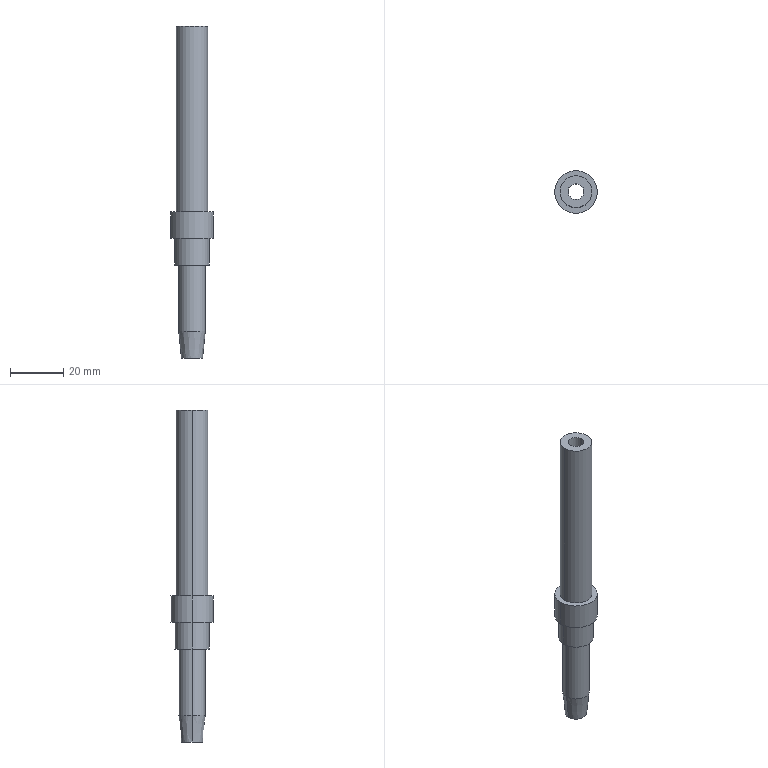Part | SolidWorks | features ICE 3, Chamfer 1, Extrusion 1 | 1 solid | 17 faces | box 16 x 16 x 125 mm | volume 10323 mm3 | cylinder 10 | plane 5 | cone 2 | commonest cylinder face diameters 6 x2 10 x2 12 x2 13 x2 16 x2
STEP:
#1=CARTESIAN_POINT('',(-4.,0.,0.));
#2=VERTEX_POINT('',#1);
#3=CARTESIAN_POINT('',(4.,0.,0.));
#4=VERTEX_POINT('',#3);
#5=CARTESIAN_POINT('',(0.,0.,0.));
#6=DIRECTION('',(0.,0.,-1.));
#7=DIRECTION('',(1.,0.,0.));
#8=AXIS2_PLACEMENT_3D('',#5,#6,#7);
#9=CIRCLE('',#8,4.);
#10=EDGE_CURVE('',#2,#4,#9,.T.);
#11=ORIENTED_EDGE('',*,*,#10,.F.);
#12=CARTESIAN_POINT('',(-5.,0.,10.));
#13=VERTEX_POINT('',#12);
#14=CARTESIAN_POINT('',(-5.,0.,10.));
#15=DIRECTION('',(-0.0995,0.,0.995));
#16=VECTOR('',#15,1000.);
#17=LINE('',#14,#16);
#18=EDGE_CURVE('',#2,#13,#17,.T.);
#19=ORIENTED_EDGE('',*,*,#18,.T.);
#20=CARTESIAN_POINT('',(5.,0.,10.));
#21=VERTEX_POINT('',#20);
#22=CARTESIAN_POINT('',(0.,0.,10.));
#23=DIRECTION('',(0.,0.,1.));
#24=DIRECTION('',(1.,0.,0.));
#25=AXIS2_PLACEMENT_3D('',#22,#23,#24);
#26=CIRCLE('',#25,5.);
#27=EDGE_CURVE('',#21,#13,#26,.T.);
#28=ORIENTED_EDGE('',*,*,#27,.F.);
#29=CARTESIAN_POINT('',(5.,0.,10.));
#30=DIRECTION('',(0.0995,0.,0.995));
#31=VECTOR('',#30,1000.);
#32=LINE('',#29,#31);
#33=EDGE_CURVE('',#4,#21,#32,.T.);
#34=ORIENTED_EDGE('',*,*,#33,.F.);
#35=EDGE_LOOP('',(#11,#19,#28,#34));
#36=FACE_OUTER_BOUND('',#35,.T.);
#37=CARTESIAN_POINT('',(0.,0.,10.));
#38=DIRECTION('',(0.,0.,1.));
#39=DIRECTION('',(1.,0.,0.));
#40=AXIS2_PLACEMENT_3D('',#37,#38,#39);
#41=CONICAL_SURFACE('',#40,5.,0.09967);
#42=ADVANCED_FACE('',(#36),#41,.T.);
#43=CARTESIAN_POINT('',(6.,0.,125.));
#44=VERTEX_POINT('',#43);
#45=CARTESIAN_POINT('',(-6.,0.,125.));
#46=VERTEX_POINT('',#45);
#47=CARTESIAN_POINT('',(0.,0.,125.));
#48=DIRECTION('',(0.,0.,1.));
#49=DIRECTION('',(1.,0.,0.));
#50=AXIS2_PLACEMENT_3D('',#47,#48,#49);
#51=CIRCLE('',#50,6.);
#52=EDGE_CURVE('',#44,#46,#51,.T.);
#53=ORIENTED_EDGE('',*,*,#52,.F.);
#54=CARTESIAN_POINT('',(6.,0.,55.));
#55=VERTEX_POINT('',#54);
#56=CARTESIAN_POINT('',(6.,0.,125.));
#57=DIRECTION('',(0.,0.,-1.));
#58=VECTOR('',#57,1000.);
#59=LINE('',#56,#58);
#60=EDGE_CURVE('',#44,#55,#59,.T.);
#61=ORIENTED_EDGE('',*,*,#60,.T.);
#62=CARTESIAN_POINT('',(-6.,0.,55.));
#63=VERTEX_POINT('',#62);
#64=CARTESIAN_POINT('',(0.,0.,55.));
#65=DIRECTION('',(0.,0.,1.));
#66=DIRECTION('',(1.,0.,0.));
#67=AXIS2_PLACEMENT_3D('',#64,#65,#66);
#68=CIRCLE('',#67,6.);
#69=EDGE_CURVE('',#55,#63,#68,.T.);
#70=ORIENTED_EDGE('',*,*,#69,.T.);
#71=CARTESIAN_POINT('',(-6.,0.,125.));
#72=DIRECTION('',(0.,0.,-1.));
#73=VECTOR('',#72,1000.);
#74=LINE('',#71,#73);
#75=EDGE_CURVE('',#46,#63,#74,.T.);
#76=ORIENTED_EDGE('',*,*,#75,.F.);
#77=EDGE_LOOP('',(#53,#61,#70,#76));
#78=FACE_OUTER_BOUND('',#77,.T.);
#79=CARTESIAN_POINT('',(0.,0.,125.));
#80=DIRECTION('',(0.,0.,-1.));
#81=DIRECTION('',(-1.,0.,0.));
#82=AXIS2_PLACEMENT_3D('',#79,#80,#81);
#83=CYLINDRICAL_SURFACE('',#82,6.);
#84=ADVANCED_FACE('',(#78),#83,.T.);
#85=CARTESIAN_POINT('',(8.,0.,55.));
#86=VERTEX_POINT('',#85);
#87=CARTESIAN_POINT('',(-8.,0.,55.));
#88=VERTEX_POINT('',#87);
#89=CARTESIAN_POINT('',(0.,0.,55.));
#90=DIRECTION('',(0.,0.,1.));
#91=DIRECTION('',(1.,0.,0.));
#92=AXIS2_PLACEMENT_3D('',#89,#90,#91);
#93=CIRCLE('',#92,8.);
#94=EDGE_CURVE('',#86,#88,#93,.T.);
#95=ORIENTED_EDGE('',*,*,#94,.F.);
#96=CARTESIAN_POINT('',(8.,0.,45.));
#97=VERTEX_POINT('',#96);
#98=CARTESIAN_POINT('',(8.,0.,55.));
#99=DIRECTION('',(0.,0.,-1.));
#100=VECTOR('',#99,1000.);
#101=LINE('',#98,#100);
#102=EDGE_CURVE('',#86,#97,#101,.T.);
#103=ORIENTED_EDGE('',*,*,#102,.T.);
#104=CARTESIAN_POINT('',(-8.,0.,45.));
#105=VERTEX_POINT('',#104);
#106=CARTESIAN_POINT('',(0.,0.,45.));
#107=DIRECTION('',(0.,0.,1.));
#108=DIRECTION('',(1.,0.,0.));
#109=AXIS2_PLACEMENT_3D('',#106,#107,#108);
#110=CIRCLE('',#109,8.);
#111=EDGE_CURVE('',#97,#105,#110,.T.);
#112=ORIENTED_EDGE('',*,*,#111,.T.);
#113=CARTESIAN_POINT('',(-8.,0.,55.));
#114=DIRECTION('',(0.,0.,-1.));
#115=VECTOR('',#114,1000.);
#116=LINE('',#113,#115);
#117=EDGE_CURVE('',#88,#105,#116,.T.);
#118=ORIENTED_EDGE('',*,*,#117,.F.);
#119=EDGE_LOOP('',(#95,#103,#112,#118));
#120=FACE_OUTER_BOUND('',#119,.T.);
#121=CARTESIAN_POINT('',(0.,0.,55.));
#122=DIRECTION('',(0.,0.,-1.));
#123=DIRECTION('',(-1.,0.,0.));
#124=AXIS2_PLACEMENT_3D('',#121,#122,#123);
#125=CYLINDRICAL_SURFACE('',#124,8.);
#126=ADVANCED_FACE('',(#120),#125,.T.);
#127=CARTESIAN_POINT('',(6.5,0.,45.));
#128=VERTEX_POINT('',#127);
#129=CARTESIAN_POINT('',(-6.5,0.,45.));
#130=VERTEX_POINT('',#129);
#131=CARTESIAN_POINT('',(0.,0.,45.));
#132=DIRECTION('',(0.,0.,1.));
#133=DIRECTION('',(1.,0.,0.));
#134=AXIS2_PLACEMENT_3D('',#131,#132,#133);
#135=CIRCLE('',#134,6.5);
#136=EDGE_CURVE('',#128,#130,#135,.T.);
#137=ORIENTED_EDGE('',*,*,#136,.F.);
#138=CARTESIAN_POINT('',(6.5,0.,35.));
#139=VERTEX_POINT('',#138);
#140=CARTESIAN_POINT('',(6.5,0.,45.));
#141=DIRECTION('',(0.,0.,-1.));
#142=VECTOR('',#141,1000.);
#143=LINE('',#140,#142);
#144=EDGE_CURVE('',#128,#139,#143,.T.);
#145=ORIENTED_EDGE('',*,*,#144,.T.);
#146=CARTESIAN_POINT('',(-6.5,0.,35.));
#147=VERTEX_POINT('',#146);
#148=CARTESIAN_POINT('',(0.,0.,35.));
#149=DIRECTION('',(0.,0.,1.));
#150=DIRECTION('',(1.,0.,0.));
#151=AXIS2_PLACEMENT_3D('',#148,#149,#150);
#152=CIRCLE('',#151,6.5);
#153=EDGE_CURVE('',#139,#147,#152,.T.);
#154=ORIENTED_EDGE('',*,*,#153,.T.);
#155=CARTESIAN_POINT('',(-6.5,0.,45.));
#156=DIRECTION('',(0.,0.,-1.));
#157=VECTOR('',#156,1000.);
#158=LINE('',#155,#157);
#159=EDGE_CURVE('',#130,#147,#158,.T.);
#160=ORIENTED_EDGE('',*,*,#159,.F.);
#161=EDGE_LOOP('',(#137,#145,#154,#160));
#162=FACE_OUTER_BOUND('',#161,.T.);
#163=CARTESIAN_POINT('',(0.,0.,45.));
#164=DIRECTION('',(0.,0.,-1.));
#165=DIRECTION('',(-1.,0.,0.));
#166=AXIS2_PLACEMENT_3D('',#163,#164,#165);
#167=CYLINDRICAL_SURFACE('',#166,6.5);
#168=ADVANCED_FACE('',(#162),#167,.T.);
#169=CARTESIAN_POINT('',(-3.,0.,125.));
#170=VERTEX_POINT('',#169);
#171=CARTESIAN_POINT('',(3.,0.,125.));
#172=VERTEX_POINT('',#171);
#173=CARTESIAN_POINT('',(0.,0.,125.));
#174=DIRECTION('',(0.,0.,1.));
#175=DIRECTION('',(1.,0.,0.));
#176=AXIS2_PLACEMENT_3D('',#173,#174,#175);
#177=CIRCLE('',#176,3.);
#178=EDGE_CURVE('',#170,#172,#177,.T.);
#179=ORIENTED_EDGE('',*,*,#178,.T.);
#180=CARTESIAN_POINT('',(3.,0.,0.));
#181=VERTEX_POINT('',#180);
#182=CARTESIAN_POINT('',(3.,0.,35.));
#183=DIRECTION('',(0.,0.,-1.));
#184=VECTOR('',#183,1000.);
#185=LINE('',#182,#184);
#186=EDGE_CURVE('',#172,#181,#185,.T.);
#187=ORIENTED_EDGE('',*,*,#186,.T.);
#188=CARTESIAN_POINT('',(-3.,0.,0.));
#189=VERTEX_POINT('',#188);
#190=CARTESIAN_POINT('',(0.,0.,0.));
#191=DIRECTION('',(0.,0.,1.));
#192=DIRECTION('',(1.,0.,0.));
#193=AXIS2_PLACEMENT_3D('',#190,#191,#192);
#194=CIRCLE('',#193,3.);
#195=EDGE_CURVE('',#189,#181,#194,.T.);
#196=ORIENTED_EDGE('',*,*,#195,.F.);
#197=CARTESIAN_POINT('',(-3.,0.,35.));
#198=DIRECTION('',(0.,0.,-1.));
#199=VECTOR('',#198,1000.);
#200=LINE('',#197,#199);
#201=EDGE_CURVE('',#170,#189,#200,.T.);
#202=ORIENTED_EDGE('',*,*,#201,.F.);
#203=EDGE_LOOP('',(#179,#187,#196,#202));
#204=FACE_OUTER_BOUND('',#203,.T.);
#205=CARTESIAN_POINT('',(0.,0.,35.));
#206=DIRECTION('',(0.,0.,-1.));
#207=DIRECTION('',(-1.,0.,0.));
#208=AXIS2_PLACEMENT_3D('',#205,#206,#207);
#209=CYLINDRICAL_SURFACE('',#208,3.);
#210=ADVANCED_FACE('',(#204),#209,.F.);
#211=CARTESIAN_POINT('',(5.,0.,35.));
#212=VERTEX_POINT('',#211);
#213=CARTESIAN_POINT('',(-5.,0.,35.));
#214=VERTEX_POINT('',#213);
#215=CARTESIAN_POINT('',(0.,0.,35.));
#216=DIRECTION('',(0.,0.,1.));
#217=DIRECTION('',(1.,0.,0.));
#218=AXIS2_PLACEMENT_3D('',#215,#216,#217);
#219=CIRCLE('',#218,5.);
#220=EDGE_CURVE('',#212,#214,#219,.T.);
#221=ORIENTED_EDGE('',*,*,#220,.F.);
#222=CARTESIAN_POINT('',(5.,0.,35.));
#223=DIRECTION('',(0.,0.,-1.));
#224=VECTOR('',#223,1000.);
#225=LINE('',#222,#224);
#226=EDGE_CURVE('',#212,#21,#225,.T.);
#227=ORIENTED_EDGE('',*,*,#226,.T.);
#228=ORIENTED_EDGE('',*,*,#27,.T.);
#229=CARTESIAN_POINT('',(-5.,0.,35.));
#230=DIRECTION('',(0.,0.,-1.));
#231=VECTOR('',#230,1000.);
#232=LINE('',#229,#231);
#233=EDGE_CURVE('',#214,#13,#232,.T.);
#234=ORIENTED_EDGE('',*,*,#233,.F.);
#235=EDGE_LOOP('',(#221,#227,#228,#234));
#236=FACE_OUTER_BOUND('',#235,.T.);
#237=CARTESIAN_POINT('',(0.,0.,35.));
#238=DIRECTION('',(0.,0.,-1.));
#239=DIRECTION('',(-1.,0.,0.));
#240=AXIS2_PLACEMENT_3D('',#237,#238,#239);
#241=CYLINDRICAL_SURFACE('',#240,5.);
#242=ADVANCED_FACE('',(#236),#241,.T.);
#243=CARTESIAN_POINT('',(0.,0.,0.));
#244=DIRECTION('',(0.,0.,-1.));
#245=DIRECTION('',(1.,0.,0.));
#246=AXIS2_PLACEMENT_3D('',#243,#244,#245);
#247=CIRCLE('',#246,4.);
#248=EDGE_CURVE('',#4,#2,#247,.T.);
#249=ORIENTED_EDGE('',*,*,#248,.T.);
#250=ORIENTED_EDGE('',*,*,#10,.T.);
#251=EDGE_LOOP('',(#249,#250));
#252=FACE_OUTER_BOUND('',#251,.T.);
#253=ORIENTED_EDGE('',*,*,#195,.T.);
#254=CARTESIAN_POINT('',(0.,0.,0.));
#255=DIRECTION('',(0.,0.,1.));
#256=DIRECTION('',(1.,0.,0.));
#257=AXIS2_PLACEMENT_3D('',#254,#255,#256);
#258=CIRCLE('',#257,3.);
#259=EDGE_CURVE('',#181,#189,#258,.T.);
#260=ORIENTED_EDGE('',*,*,#259,.T.);
#261=EDGE_LOOP('',(#253,#260));
#262=FACE_BOUND('',#261,.T.);
#263=CARTESIAN_POINT('',(0.,0.,0.));
#264=DIRECTION('',(0.,0.,1.));
#265=DIRECTION('',(1.,0.,0.));
#266=AXIS2_PLACEMENT_3D('',#263,#264,#265);
#267=PLANE('',#266);
#268=ADVANCED_FACE('',(#252,#262),#267,.F.);
#269=ORIENTED_EDGE('',*,*,#226,.F.);
#270=CARTESIAN_POINT('',(0.,0.,35.));
#271=DIRECTION('',(0.,0.,1.));
#272=DIRECTION('',(1.,0.,0.));
#273=AXIS2_PLACEMENT_3D('',#270,#271,#272);
#274=CIRCLE('',#273,5.);
#275=EDGE_CURVE('',#214,#212,#274,.T.);
#276=ORIENTED_EDGE('',*,*,#275,.F.);
#277=ORIENTED_EDGE('',*,*,#233,.T.);
#278=CARTESIAN_POINT('',(0.,0.,10.));
#279=DIRECTION('',(0.,0.,1.));
#280=DIRECTION('',(1.,0.,0.));
#281=AXIS2_PLACEMENT_3D('',#278,#279,#280);
#282=CIRCLE('',#281,5.);
#283=EDGE_CURVE('',#13,#21,#282,.T.);
#284=ORIENTED_EDGE('',*,*,#283,.T.);
#285=EDGE_LOOP('',(#269,#276,#277,#284));
#286=FACE_OUTER_BOUND('',#285,.T.);
#287=CARTESIAN_POINT('',(0.,0.,35.));
#288=DIRECTION('',(0.,0.,-1.));
#289=DIRECTION('',(-1.,0.,0.));
#290=AXIS2_PLACEMENT_3D('',#287,#288,#289);
#291=CYLINDRICAL_SURFACE('',#290,5.);
#292=ADVANCED_FACE('',(#286),#291,.T.);
#293=ORIENTED_EDGE('',*,*,#186,.F.);
#294=CARTESIAN_POINT('',(0.,0.,125.));
#295=DIRECTION('',(0.,0.,1.));
#296=DIRECTION('',(1.,0.,0.));
#297=AXIS2_PLACEMENT_3D('',#294,#295,#296);
#298=CIRCLE('',#297,3.);
#299=EDGE_CURVE('',#172,#170,#298,.T.);
#300=ORIENTED_EDGE('',*,*,#299,.T.);
#301=ORIENTED_EDGE('',*,*,#201,.T.);
#302=ORIENTED_EDGE('',*,*,#259,.F.);
#303=EDGE_LOOP('',(#293,#300,#301,#302));
#304=FACE_OUTER_BOUND('',#303,.T.);
#305=CARTESIAN_POINT('',(0.,0.,35.));
#306=DIRECTION('',(0.,0.,-1.));
#307=DIRECTION('',(-1.,0.,0.));
#308=AXIS2_PLACEMENT_3D('',#305,#306,#307);
#309=CYLINDRICAL_SURFACE('',#308,3.);
#310=ADVANCED_FACE('',(#304),#309,.F.);
#311=ORIENTED_EDGE('',*,*,#275,.T.);
#312=ORIENTED_EDGE('',*,*,#220,.T.);
#313=EDGE_LOOP('',(#311,#312));
#314=FACE_BOUND('',#313,.T.);
#315=CARTESIAN_POINT('',(0.,0.,35.));
#316=DIRECTION('',(0.,0.,1.));
#317=DIRECTION('',(1.,0.,0.));
#318=AXIS2_PLACEMENT_3D('',#315,#316,#317);
#319=CIRCLE('',#318,6.5);
#320=EDGE_CURVE('',#147,#139,#319,.T.);
#321=ORIENTED_EDGE('',*,*,#320,.F.);
#322=ORIENTED_EDGE('',*,*,#153,.F.);
#323=EDGE_LOOP('',(#321,#322));
#324=FACE_OUTER_BOUND('',#323,.T.);
#325=CARTESIAN_POINT('',(0.,0.,35.));
#326=DIRECTION('',(0.,0.,1.));
#327=DIRECTION('',(1.,0.,0.));
#328=AXIS2_PLACEMENT_3D('',#325,#326,#327);
#329=PLANE('',#328);
#330=ADVANCED_FACE('',(#314,#324),#329,.F.);
#331=ORIENTED_EDGE('',*,*,#144,.F.);
#332=CARTESIAN_POINT('',(0.,0.,45.));
#333=DIRECTION('',(0.,0.,1.));
#334=DIRECTION('',(1.,0.,0.));
#335=AXIS2_PLACEMENT_3D('',#332,#333,#334);
#336=CIRCLE('',#335,6.5);
#337=EDGE_CURVE('',#130,#128,#336,.T.);
#338=ORIENTED_EDGE('',*,*,#337,.F.);
#339=ORIENTED_EDGE('',*,*,#159,.T.);
#340=ORIENTED_EDGE('',*,*,#320,.T.);
#341=EDGE_LOOP('',(#331,#338,#339,#340));
#342=FACE_OUTER_BOUND('',#341,.T.);
#343=CARTESIAN_POINT('',(0.,0.,45.));
#344=DIRECTION('',(0.,0.,-1.));
#345=DIRECTION('',(-1.,0.,0.));
#346=AXIS2_PLACEMENT_3D('',#343,#344,#345);
#347=CYLINDRICAL_SURFACE('',#346,6.5);
#348=ADVANCED_FACE('',(#342),#347,.T.);
#349=CARTESIAN_POINT('',(0.,0.,55.));
#350=DIRECTION('',(0.,0.,1.));
#351=DIRECTION('',(1.,0.,0.));
#352=AXIS2_PLACEMENT_3D('',#349,#350,#351);
#353=CIRCLE('',#352,6.);
#354=EDGE_CURVE('',#63,#55,#353,.T.);
#355=ORIENTED_EDGE('',*,*,#354,.F.);
#356=ORIENTED_EDGE('',*,*,#69,.F.);
#357=EDGE_LOOP('',(#355,#356));
#358=FACE_BOUND('',#357,.T.);
#359=CARTESIAN_POINT('',(0.,0.,55.));
#360=DIRECTION('',(0.,0.,1.));
#361=DIRECTION('',(1.,0.,0.));
#362=AXIS2_PLACEMENT_3D('',#359,#360,#361);
#363=CIRCLE('',#362,8.);
#364=EDGE_CURVE('',#88,#86,#363,.T.);
#365=ORIENTED_EDGE('',*,*,#364,.T.);
#366=ORIENTED_EDGE('',*,*,#94,.T.);
#367=EDGE_LOOP('',(#365,#366));
#368=FACE_OUTER_BOUND('',#367,.T.);
#369=CARTESIAN_POINT('',(0.,0.,55.));
#370=DIRECTION('',(0.,0.,1.));
#371=DIRECTION('',(1.,0.,0.));
#372=AXIS2_PLACEMENT_3D('',#369,#370,#371);
#373=PLANE('',#372);
#374=ADVANCED_FACE('',(#358,#368),#373,.T.);
#375=ORIENTED_EDGE('',*,*,#337,.T.);
#376=ORIENTED_EDGE('',*,*,#136,.T.);
#377=EDGE_LOOP('',(#375,#376));
#378=FACE_BOUND('',#377,.T.);
#379=CARTESIAN_POINT('',(0.,0.,45.));
#380=DIRECTION('',(0.,0.,1.));
#381=DIRECTION('',(1.,0.,0.));
#382=AXIS2_PLACEMENT_3D('',#379,#380,#381);
#383=CIRCLE('',#382,8.);
#384=EDGE_CURVE('',#105,#97,#383,.T.);
#385=ORIENTED_EDGE('',*,*,#384,.F.);
#386=ORIENTED_EDGE('',*,*,#111,.F.);
#387=EDGE_LOOP('',(#385,#386));
#388=FACE_OUTER_BOUND('',#387,.T.);
#389=CARTESIAN_POINT('',(0.,0.,45.));
#390=DIRECTION('',(0.,0.,1.));
#391=DIRECTION('',(1.,0.,0.));
#392=AXIS2_PLACEMENT_3D('',#389,#390,#391);
#393=PLANE('',#392);
#394=ADVANCED_FACE('',(#378,#388),#393,.F.);
#395=ORIENTED_EDGE('',*,*,#102,.F.);
#396=ORIENTED_EDGE('',*,*,#364,.F.);
#397=ORIENTED_EDGE('',*,*,#117,.T.);
#398=ORIENTED_EDGE('',*,*,#384,.T.);
#399=EDGE_LOOP('',(#395,#396,#397,#398));
#400=FACE_OUTER_BOUND('',#399,.T.);
#401=CARTESIAN_POINT('',(0.,0.,55.));
#402=DIRECTION('',(0.,0.,-1.));
#403=DIRECTION('',(-1.,0.,0.));
#404=AXIS2_PLACEMENT_3D('',#401,#402,#403);
#405=CYLINDRICAL_SURFACE('',#404,8.);
#406=ADVANCED_FACE('',(#400),#405,.T.);
#407=CARTESIAN_POINT('',(0.,0.,125.));
#408=DIRECTION('',(0.,0.,1.));
#409=DIRECTION('',(1.,0.,0.));
#410=AXIS2_PLACEMENT_3D('',#407,#408,#409);
#411=CIRCLE('',#410,6.);
#412=EDGE_CURVE('',#46,#44,#411,.T.);
#413=ORIENTED_EDGE('',*,*,#412,.T.);
#414=ORIENTED_EDGE('',*,*,#52,.T.);
#415=EDGE_LOOP('',(#413,#414));
#416=FACE_OUTER_BOUND('',#415,.T.);
#417=ORIENTED_EDGE('',*,*,#178,.F.);
#418=ORIENTED_EDGE('',*,*,#299,.F.);
#419=EDGE_LOOP('',(#417,#418));
#420=FACE_BOUND('',#419,.T.);
#421=CARTESIAN_POINT('',(0.,0.,125.));
#422=DIRECTION('',(0.,0.,1.));
#423=DIRECTION('',(1.,0.,0.));
#424=AXIS2_PLACEMENT_3D('',#421,#422,#423);
#425=PLANE('',#424);
#426=ADVANCED_FACE('',(#416,#420),#425,.T.);
#427=ORIENTED_EDGE('',*,*,#60,.F.);
#428=ORIENTED_EDGE('',*,*,#412,.F.);
#429=ORIENTED_EDGE('',*,*,#75,.T.);
#430=ORIENTED_EDGE('',*,*,#354,.T.);
#431=EDGE_LOOP('',(#427,#428,#429,#430));
#432=FACE_OUTER_BOUND('',#431,.T.);
#433=CARTESIAN_POINT('',(0.,0.,125.));
#434=DIRECTION('',(0.,0.,-1.));
#435=DIRECTION('',(-1.,0.,0.));
#436=AXIS2_PLACEMENT_3D('',#433,#434,#435);
#437=CYLINDRICAL_SURFACE('',#436,6.);
#438=ADVANCED_FACE('',(#432),#437,.T.);
#439=ORIENTED_EDGE('',*,*,#18,.F.);
#440=ORIENTED_EDGE('',*,*,#248,.F.);
#441=ORIENTED_EDGE('',*,*,#33,.T.);
#442=ORIENTED_EDGE('',*,*,#283,.F.);
#443=EDGE_LOOP('',(#439,#440,#441,#442));
#444=FACE_OUTER_BOUND('',#443,.T.);
#445=CARTESIAN_POINT('',(0.,0.,10.));
#446=DIRECTION('',(0.,0.,1.));
#447=DIRECTION('',(1.,0.,0.));
#448=AXIS2_PLACEMENT_3D('',#445,#446,#447);
#449=CONICAL_SURFACE('',#448,5.,0.09967);
#450=ADVANCED_FACE('',(#444),#449,.T.);
#451=CLOSED_SHELL('',(#42,#84,#126,#168,#210,#242,#268,#292,#310,#330,#348,#374,#394,#406,#426,#438,#450));
#452=MANIFOLD_SOLID_BREP('',#451);
#453=CARTESIAN_POINT('',(0.,0.,0.));
#454=DIRECTION('',(0.,0.,1.));
#455=DIRECTION('',(1.,0.,0.));
#456=AXIS2_PLACEMENT_3D('',#453,#454,#455);
#457=(LENGTH_UNIT()NAMED_UNIT(*)SI_UNIT(.MILLI.,.METRE.));
#458=UNCERTAINTY_MEASURE_WITH_UNIT(LENGTH_MEASURE(0.00001),#457,'','');
#459=(NAMED_UNIT(*)PLANE_ANGLE_UNIT()SI_UNIT($,.RADIAN.));
#460=(NAMED_UNIT(*)SI_UNIT($,.STERADIAN.)SOLID_ANGLE_UNIT());
#461=(GEOMETRIC_REPRESENTATION_CONTEXT(3)GLOBAL_UNCERTAINTY_ASSIGNED_CONTEXT((#458))GLOBAL_UNIT_ASSIGNED_CONTEXT((#457,#459,#460))REPRESENTATION_CONTEXT('',''));
#462=ADVANCED_BREP_SHAPE_REPRESENTATION('',(#452,#456),#461);